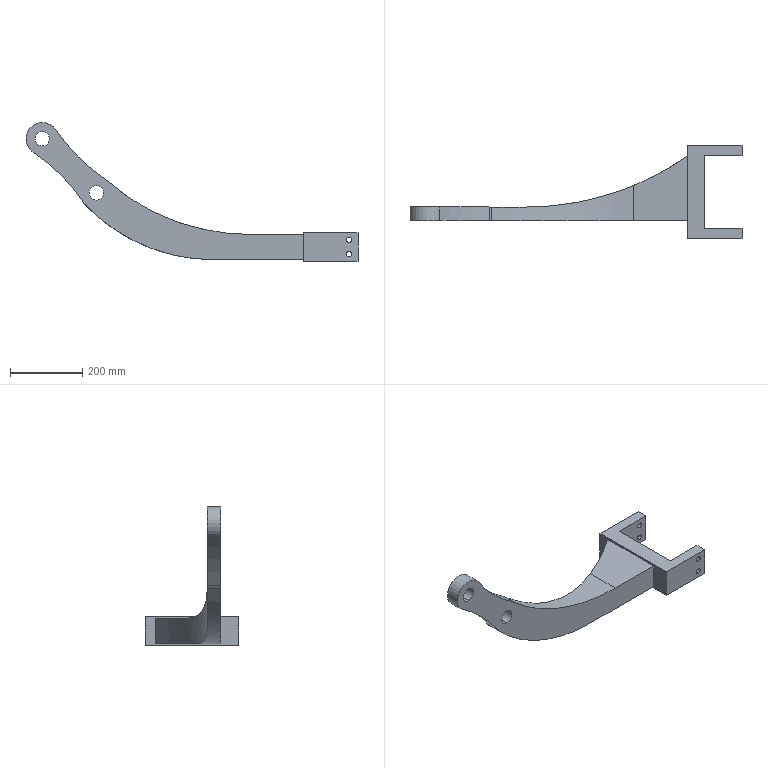Part | SolidWorks | features ICE 3, Cut 1, Extrusion 1, MirrorSolid 1 | 1 solid | 34 faces | box 920 x 260 x 385 mm | volume 5479591 mm3 | cylinder 20 | plane 14 | commonest cylinder face diameters 15 x8 40 x4 90 x3 1000 x2 984.464 x1 1199 x1
STEP:
#1=CARTESIAN_POINT('',(50.,-130.,12.5));
#2=VERTEX_POINT('',#1);
#3=CARTESIAN_POINT('',(50.,-130.,27.5));
#4=VERTEX_POINT('',#3);
#5=CARTESIAN_POINT('',(50.,-130.,20.));
#6=DIRECTION('',(0.,-1.,0.));
#7=DIRECTION('',(0.,0.,-1.));
#8=AXIS2_PLACEMENT_3D('',#5,#6,#7);
#9=CIRCLE('',#8,7.5);
#10=EDGE_CURVE('',#2,#4,#9,.T.);
#11=ORIENTED_EDGE('',*,*,#10,.T.);
#12=CARTESIAN_POINT('',(50.,-100.,27.5));
#13=VERTEX_POINT('',#12);
#14=CARTESIAN_POINT('',(50.,-130.,27.5));
#15=DIRECTION('',(0.,1.,0.));
#16=VECTOR('',#15,1000.);
#17=LINE('',#14,#16);
#18=EDGE_CURVE('',#4,#13,#17,.T.);
#19=ORIENTED_EDGE('',*,*,#18,.T.);
#20=CARTESIAN_POINT('',(50.,-100.,12.5));
#21=VERTEX_POINT('',#20);
#22=CARTESIAN_POINT('',(50.,-100.,20.));
#23=DIRECTION('',(0.,1.,0.));
#24=DIRECTION('',(0.,0.,1.));
#25=AXIS2_PLACEMENT_3D('',#22,#23,#24);
#26=CIRCLE('',#25,7.5);
#27=EDGE_CURVE('',#13,#21,#26,.T.);
#28=ORIENTED_EDGE('',*,*,#27,.T.);
#29=CARTESIAN_POINT('',(50.,-130.,12.5));
#30=DIRECTION('',(0.,1.,0.));
#31=VECTOR('',#30,1000.);
#32=LINE('',#29,#31);
#33=EDGE_CURVE('',#2,#21,#32,.T.);
#34=ORIENTED_EDGE('',*,*,#33,.F.);
#35=EDGE_LOOP('',(#11,#19,#28,#34));
#36=FACE_OUTER_BOUND('',#35,.T.);
#37=CARTESIAN_POINT('',(50.,-130.,20.));
#38=DIRECTION('',(0.,1.,0.));
#39=DIRECTION('',(0.,0.,-1.));
#40=AXIS2_PLACEMENT_3D('',#37,#38,#39);
#41=CYLINDRICAL_SURFACE('',#40,7.5);
#42=ADVANCED_FACE('',(#36),#41,.F.);
#43=CARTESIAN_POINT('',(50.,-130.,-27.5));
#44=VERTEX_POINT('',#43);
#45=CARTESIAN_POINT('',(50.,-130.,-12.5));
#46=VERTEX_POINT('',#45);
#47=CARTESIAN_POINT('',(50.,-130.,-20.));
#48=DIRECTION('',(0.,-1.,0.));
#49=DIRECTION('',(0.,0.,-1.));
#50=AXIS2_PLACEMENT_3D('',#47,#48,#49);
#51=CIRCLE('',#50,7.5);
#52=EDGE_CURVE('',#44,#46,#51,.T.);
#53=ORIENTED_EDGE('',*,*,#52,.T.);
#54=CARTESIAN_POINT('',(50.,-100.,-12.5));
#55=VERTEX_POINT('',#54);
#56=CARTESIAN_POINT('',(50.,-130.,-12.5));
#57=DIRECTION('',(0.,1.,0.));
#58=VECTOR('',#57,1000.);
#59=LINE('',#56,#58);
#60=EDGE_CURVE('',#46,#55,#59,.T.);
#61=ORIENTED_EDGE('',*,*,#60,.T.);
#62=CARTESIAN_POINT('',(50.,-100.,-27.5));
#63=VERTEX_POINT('',#62);
#64=CARTESIAN_POINT('',(50.,-100.,-20.));
#65=DIRECTION('',(0.,1.,0.));
#66=DIRECTION('',(0.,0.,1.));
#67=AXIS2_PLACEMENT_3D('',#64,#65,#66);
#68=CIRCLE('',#67,7.5);
#69=EDGE_CURVE('',#55,#63,#68,.T.);
#70=ORIENTED_EDGE('',*,*,#69,.T.);
#71=CARTESIAN_POINT('',(50.,-130.,-27.5));
#72=DIRECTION('',(0.,1.,0.));
#73=VECTOR('',#72,1000.);
#74=LINE('',#71,#73);
#75=EDGE_CURVE('',#44,#63,#74,.T.);
#76=ORIENTED_EDGE('',*,*,#75,.F.);
#77=EDGE_LOOP('',(#53,#61,#70,#76));
#78=FACE_OUTER_BOUND('',#77,.T.);
#79=CARTESIAN_POINT('',(50.,-130.,-20.));
#80=DIRECTION('',(0.,1.,0.));
#81=DIRECTION('',(0.,0.,-1.));
#82=AXIS2_PLACEMENT_3D('',#79,#80,#81);
#83=CYLINDRICAL_SURFACE('',#82,7.5);
#84=ADVANCED_FACE('',(#78),#83,.F.);
#85=CARTESIAN_POINT('',(50.,100.,12.5));
#86=VERTEX_POINT('',#85);
#87=CARTESIAN_POINT('',(50.,100.,27.5));
#88=VERTEX_POINT('',#87);
#89=CARTESIAN_POINT('',(50.,100.,20.));
#90=DIRECTION('',(0.,-1.,0.));
#91=DIRECTION('',(0.,0.,-1.));
#92=AXIS2_PLACEMENT_3D('',#89,#90,#91);
#93=CIRCLE('',#92,7.5);
#94=EDGE_CURVE('',#86,#88,#93,.T.);
#95=ORIENTED_EDGE('',*,*,#94,.T.);
#96=CARTESIAN_POINT('',(50.,130.,27.5));
#97=VERTEX_POINT('',#96);
#98=CARTESIAN_POINT('',(50.,-130.,27.5));
#99=DIRECTION('',(0.,1.,0.));
#100=VECTOR('',#99,1000.);
#101=LINE('',#98,#100);
#102=EDGE_CURVE('',#88,#97,#101,.T.);
#103=ORIENTED_EDGE('',*,*,#102,.T.);
#104=CARTESIAN_POINT('',(50.,130.,12.5));
#105=VERTEX_POINT('',#104);
#106=CARTESIAN_POINT('',(50.,130.,20.));
#107=DIRECTION('',(0.,-1.,0.));
#108=DIRECTION('',(0.,0.,-1.));
#109=AXIS2_PLACEMENT_3D('',#106,#107,#108);
#110=CIRCLE('',#109,7.5);
#111=EDGE_CURVE('',#105,#97,#110,.T.);
#112=ORIENTED_EDGE('',*,*,#111,.F.);
#113=CARTESIAN_POINT('',(50.,-130.,12.5));
#114=DIRECTION('',(0.,1.,0.));
#115=VECTOR('',#114,1000.);
#116=LINE('',#113,#115);
#117=EDGE_CURVE('',#86,#105,#116,.T.);
#118=ORIENTED_EDGE('',*,*,#117,.F.);
#119=EDGE_LOOP('',(#95,#103,#112,#118));
#120=FACE_OUTER_BOUND('',#119,.T.);
#121=CARTESIAN_POINT('',(50.,-130.,20.));
#122=DIRECTION('',(0.,1.,0.));
#123=DIRECTION('',(0.,0.,-1.));
#124=AXIS2_PLACEMENT_3D('',#121,#122,#123);
#125=CYLINDRICAL_SURFACE('',#124,7.5);
#126=ADVANCED_FACE('',(#120),#125,.F.);
#127=CARTESIAN_POINT('',(50.,100.,-27.5));
#128=VERTEX_POINT('',#127);
#129=CARTESIAN_POINT('',(50.,100.,-12.5));
#130=VERTEX_POINT('',#129);
#131=CARTESIAN_POINT('',(50.,100.,-20.));
#132=DIRECTION('',(0.,-1.,0.));
#133=DIRECTION('',(0.,0.,-1.));
#134=AXIS2_PLACEMENT_3D('',#131,#132,#133);
#135=CIRCLE('',#134,7.5);
#136=EDGE_CURVE('',#128,#130,#135,.T.);
#137=ORIENTED_EDGE('',*,*,#136,.T.);
#138=CARTESIAN_POINT('',(50.,130.,-12.5));
#139=VERTEX_POINT('',#138);
#140=CARTESIAN_POINT('',(50.,-130.,-12.5));
#141=DIRECTION('',(0.,1.,0.));
#142=VECTOR('',#141,1000.);
#143=LINE('',#140,#142);
#144=EDGE_CURVE('',#130,#139,#143,.T.);
#145=ORIENTED_EDGE('',*,*,#144,.T.);
#146=CARTESIAN_POINT('',(50.,130.,-27.5));
#147=VERTEX_POINT('',#146);
#148=CARTESIAN_POINT('',(50.,130.,-20.));
#149=DIRECTION('',(0.,-1.,0.));
#150=DIRECTION('',(0.,0.,-1.));
#151=AXIS2_PLACEMENT_3D('',#148,#149,#150);
#152=CIRCLE('',#151,7.5);
#153=EDGE_CURVE('',#147,#139,#152,.T.);
#154=ORIENTED_EDGE('',*,*,#153,.F.);
#155=CARTESIAN_POINT('',(50.,-130.,-27.5));
#156=DIRECTION('',(0.,1.,0.));
#157=VECTOR('',#156,1000.);
#158=LINE('',#155,#157);
#159=EDGE_CURVE('',#128,#147,#158,.T.);
#160=ORIENTED_EDGE('',*,*,#159,.F.);
#161=EDGE_LOOP('',(#137,#145,#154,#160));
#162=FACE_OUTER_BOUND('',#161,.T.);
#163=CARTESIAN_POINT('',(50.,-130.,-20.));
#164=DIRECTION('',(0.,1.,0.));
#165=DIRECTION('',(0.,0.,-1.));
#166=AXIS2_PLACEMENT_3D('',#163,#164,#165);
#167=CYLINDRICAL_SURFACE('',#166,7.5);
#168=ADVANCED_FACE('',(#162),#167,.F.);
#169=CARTESIAN_POINT('',(-650.,-80.,170.));
#170=VERTEX_POINT('',#169);
#171=CARTESIAN_POINT('',(-650.,-80.,130.));
#172=VERTEX_POINT('',#171);
#173=CARTESIAN_POINT('',(-650.,-80.,150.));
#174=DIRECTION('',(0.,1.,0.));
#175=DIRECTION('',(-1.,0.,0.));
#176=AXIS2_PLACEMENT_3D('',#173,#174,#175);
#177=CIRCLE('',#176,20.);
#178=EDGE_CURVE('',#170,#172,#177,.T.);
#179=ORIENTED_EDGE('',*,*,#178,.F.);
#180=CARTESIAN_POINT('',(-650.,-41.894,170.));
#181=VERTEX_POINT('',#180);
#182=CARTESIAN_POINT('',(-650.,-100.,170.));
#183=DIRECTION('',(0.,1.,0.));
#184=VECTOR('',#183,1000.);
#185=LINE('',#182,#184);
#186=EDGE_CURVE('',#170,#181,#185,.T.);
#187=ORIENTED_EDGE('',*,*,#186,.T.);
#188=CARTESIAN_POINT('',(-650.,-41.894,130.));
#189=VERTEX_POINT('',#188);
#190=CARTESIAN_POINT('',(-650.,-41.894,150.));
#191=DIRECTION('',(0.,-1.,0.));
#192=DIRECTION('',(0.,0.,1.));
#193=AXIS2_PLACEMENT_3D('',#190,#191,#192);
#194=CIRCLE('',#193,20.);
#195=EDGE_CURVE('',#189,#181,#194,.T.);
#196=ORIENTED_EDGE('',*,*,#195,.F.);
#197=CARTESIAN_POINT('',(-650.,-100.,130.));
#198=DIRECTION('',(0.,1.,0.));
#199=VECTOR('',#198,1000.);
#200=LINE('',#197,#199);
#201=EDGE_CURVE('',#172,#189,#200,.T.);
#202=ORIENTED_EDGE('',*,*,#201,.F.);
#203=EDGE_LOOP('',(#179,#187,#196,#202));
#204=FACE_OUTER_BOUND('',#203,.T.);
#205=CARTESIAN_POINT('',(-650.,-100.,150.));
#206=DIRECTION('',(0.,1.,0.));
#207=DIRECTION('',(0.,0.,-1.));
#208=AXIS2_PLACEMENT_3D('',#205,#206,#207);
#209=CYLINDRICAL_SURFACE('',#208,20.);
#210=ADVANCED_FACE('',(#204),#209,.F.);
#211=CARTESIAN_POINT('',(-800.,-80.,320.));
#212=VERTEX_POINT('',#211);
#213=CARTESIAN_POINT('',(-800.,-80.,280.));
#214=VERTEX_POINT('',#213);
#215=CARTESIAN_POINT('',(-800.,-80.,300.));
#216=DIRECTION('',(0.,1.,0.));
#217=DIRECTION('',(-1.,0.,0.));
#218=AXIS2_PLACEMENT_3D('',#215,#216,#217);
#219=CIRCLE('',#218,20.);
#220=EDGE_CURVE('',#212,#214,#219,.T.);
#221=ORIENTED_EDGE('',*,*,#220,.F.);
#222=CARTESIAN_POINT('',(-800.,-41.894,320.));
#223=VERTEX_POINT('',#222);
#224=CARTESIAN_POINT('',(-800.,-100.,320.));
#225=DIRECTION('',(0.,1.,0.));
#226=VECTOR('',#225,1000.);
#227=LINE('',#224,#226);
#228=EDGE_CURVE('',#212,#223,#227,.T.);
#229=ORIENTED_EDGE('',*,*,#228,.T.);
#230=CARTESIAN_POINT('',(-800.,-41.894,280.));
#231=VERTEX_POINT('',#230);
#232=CARTESIAN_POINT('',(-800.,-41.894,300.));
#233=DIRECTION('',(0.,-1.,0.));
#234=DIRECTION('',(0.,0.,1.));
#235=AXIS2_PLACEMENT_3D('',#232,#233,#234);
#236=CIRCLE('',#235,20.);
#237=EDGE_CURVE('',#231,#223,#236,.T.);
#238=ORIENTED_EDGE('',*,*,#237,.F.);
#239=CARTESIAN_POINT('',(-800.,-100.,280.));
#240=DIRECTION('',(0.,1.,0.));
#241=VECTOR('',#240,1000.);
#242=LINE('',#239,#241);
#243=EDGE_CURVE('',#214,#231,#242,.T.);
#244=ORIENTED_EDGE('',*,*,#243,.F.);
#245=EDGE_LOOP('',(#221,#229,#238,#244));
#246=FACE_OUTER_BOUND('',#245,.T.);
#247=CARTESIAN_POINT('',(-800.,-100.,300.));
#248=DIRECTION('',(0.,1.,0.));
#249=DIRECTION('',(0.,0.,-1.));
#250=AXIS2_PLACEMENT_3D('',#247,#248,#249);
#251=CYLINDRICAL_SURFACE('',#250,20.);
#252=ADVANCED_FACE('',(#246),#251,.F.);
#253=CARTESIAN_POINT('',(-75.,100.,-35.));
#254=VERTEX_POINT('',#253);
#255=CARTESIAN_POINT('',(-75.,100.,35.));
#256=VERTEX_POINT('',#255);
#257=CARTESIAN_POINT('',(-75.,100.,35.));
#258=DIRECTION('',(0.,0.,1.));
#259=VECTOR('',#258,1000.);
#260=LINE('',#257,#259);
#261=EDGE_CURVE('',#254,#256,#260,.T.);
#262=ORIENTED_EDGE('',*,*,#261,.T.);
#263=CARTESIAN_POINT('',(-75.,-80.,35.));
#264=VERTEX_POINT('',#263);
#265=CARTESIAN_POINT('',(-75.,-100.,35.));
#266=DIRECTION('',(0.,1.,0.));
#267=VECTOR('',#266,1000.);
#268=LINE('',#265,#267);
#269=EDGE_CURVE('',#264,#256,#268,.T.);
#270=ORIENTED_EDGE('',*,*,#269,.F.);
#271=CARTESIAN_POINT('',(-75.,-80.,-35.));
#272=VERTEX_POINT('',#271);
#273=CARTESIAN_POINT('',(-75.,-80.,345.));
#274=DIRECTION('',(0.,0.,-1.));
#275=VECTOR('',#274,1000.);
#276=LINE('',#273,#275);
#277=EDGE_CURVE('',#264,#272,#276,.T.);
#278=ORIENTED_EDGE('',*,*,#277,.T.);
#279=CARTESIAN_POINT('',(-75.,-100.,-35.));
#280=DIRECTION('',(0.,1.,0.));
#281=VECTOR('',#280,1000.);
#282=LINE('',#279,#281);
#283=EDGE_CURVE('',#272,#254,#282,.T.);
#284=ORIENTED_EDGE('',*,*,#283,.T.);
#285=EDGE_LOOP('',(#262,#270,#278,#284));
#286=FACE_BOUND('',#285,.T.);
#287=CARTESIAN_POINT('',(-75.,130.,40.));
#288=VERTEX_POINT('',#287);
#289=CARTESIAN_POINT('',(-75.,-130.,40.));
#290=VERTEX_POINT('',#289);
#291=CARTESIAN_POINT('',(-75.,130.,40.));
#292=DIRECTION('',(0.,-1.,0.));
#293=VECTOR('',#292,1000.);
#294=LINE('',#291,#293);
#295=EDGE_CURVE('',#288,#290,#294,.T.);
#296=ORIENTED_EDGE('',*,*,#295,.F.);
#297=CARTESIAN_POINT('',(-75.,130.,-40.));
#298=VERTEX_POINT('',#297);
#299=CARTESIAN_POINT('',(-75.,130.,-40.));
#300=DIRECTION('',(0.,0.,1.));
#301=VECTOR('',#300,1000.);
#302=LINE('',#299,#301);
#303=EDGE_CURVE('',#298,#288,#302,.T.);
#304=ORIENTED_EDGE('',*,*,#303,.F.);
#305=CARTESIAN_POINT('',(-75.,-130.,-40.));
#306=VERTEX_POINT('',#305);
#307=CARTESIAN_POINT('',(-75.,130.,-40.));
#308=DIRECTION('',(0.,-1.,0.));
#309=VECTOR('',#308,1000.);
#310=LINE('',#307,#309);
#311=EDGE_CURVE('',#298,#306,#310,.T.);
#312=ORIENTED_EDGE('',*,*,#311,.T.);
#313=CARTESIAN_POINT('',(-75.,-130.,-40.));
#314=DIRECTION('',(0.,0.,1.));
#315=VECTOR('',#314,1000.);
#316=LINE('',#313,#315);
#317=EDGE_CURVE('',#306,#290,#316,.T.);
#318=ORIENTED_EDGE('',*,*,#317,.T.);
#319=EDGE_LOOP('',(#296,#304,#312,#318));
#320=FACE_OUTER_BOUND('',#319,.T.);
#321=CARTESIAN_POINT('',(-75.,130.,-40.));
#322=DIRECTION('',(1.,0.,0.));
#323=DIRECTION('',(0.,1.,0.));
#324=AXIS2_PLACEMENT_3D('',#321,#322,#323);
#325=PLANE('',#324);
#326=ADVANCED_FACE('',(#286,#320),#325,.F.);
#327=CARTESIAN_POINT('',(75.,-130.,40.));
#328=VERTEX_POINT('',#327);
#329=CARTESIAN_POINT('',(75.,-100.,40.));
#330=VERTEX_POINT('',#329);
#331=CARTESIAN_POINT('',(75.,130.,40.));
#332=DIRECTION('',(0.,1.,0.));
#333=VECTOR('',#332,1000.);
#334=LINE('',#331,#333);
#335=EDGE_CURVE('',#328,#330,#334,.T.);
#336=ORIENTED_EDGE('',*,*,#335,.F.);
#337=CARTESIAN_POINT('',(75.,-130.,-40.));
#338=VERTEX_POINT('',#337);
#339=CARTESIAN_POINT('',(75.,-130.,-40.));
#340=DIRECTION('',(0.,0.,1.));
#341=VECTOR('',#340,1000.);
#342=LINE('',#339,#341);
#343=EDGE_CURVE('',#338,#328,#342,.T.);
#344=ORIENTED_EDGE('',*,*,#343,.F.);
#345=CARTESIAN_POINT('',(75.,-100.,-40.));
#346=VERTEX_POINT('',#345);
#347=CARTESIAN_POINT('',(75.,130.,-40.));
#348=DIRECTION('',(0.,1.,0.));
#349=VECTOR('',#348,1000.);
#350=LINE('',#347,#349);
#351=EDGE_CURVE('',#338,#346,#350,.T.);
#352=ORIENTED_EDGE('',*,*,#351,.T.);
#353=CARTESIAN_POINT('',(75.,-100.,-40.));
#354=DIRECTION('',(0.,0.,-1.));
#355=VECTOR('',#354,1000.);
#356=LINE('',#353,#355);
#357=EDGE_CURVE('',#330,#346,#356,.T.);
#358=ORIENTED_EDGE('',*,*,#357,.F.);
#359=EDGE_LOOP('',(#336,#344,#352,#358));
#360=FACE_OUTER_BOUND('',#359,.T.);
#361=CARTESIAN_POINT('',(75.,130.,-40.));
#362=DIRECTION('',(-1.,0.,0.));
#363=DIRECTION('',(0.,-1.,0.));
#364=AXIS2_PLACEMENT_3D('',#361,#362,#363);
#365=PLANE('',#364);
#366=ADVANCED_FACE('',(#360),#365,.F.);
#367=CARTESIAN_POINT('',(75.,100.,-40.));
#368=VERTEX_POINT('',#367);
#369=CARTESIAN_POINT('',(75.,130.,-40.));
#370=VERTEX_POINT('',#369);
#371=CARTESIAN_POINT('',(75.,130.,-40.));
#372=DIRECTION('',(0.,1.,0.));
#373=VECTOR('',#372,1000.);
#374=LINE('',#371,#373);
#375=EDGE_CURVE('',#368,#370,#374,.T.);
#376=ORIENTED_EDGE('',*,*,#375,.T.);
#377=CARTESIAN_POINT('',(75.,130.,40.));
#378=VERTEX_POINT('',#377);
#379=CARTESIAN_POINT('',(75.,130.,-40.));
#380=DIRECTION('',(0.,0.,1.));
#381=VECTOR('',#380,1000.);
#382=LINE('',#379,#381);
#383=EDGE_CURVE('',#370,#378,#382,.T.);
#384=ORIENTED_EDGE('',*,*,#383,.T.);
#385=CARTESIAN_POINT('',(75.,100.,40.));
#386=VERTEX_POINT('',#385);
#387=CARTESIAN_POINT('',(75.,130.,40.));
#388=DIRECTION('',(0.,1.,0.));
#389=VECTOR('',#388,1000.);
#390=LINE('',#387,#389);
#391=EDGE_CURVE('',#386,#378,#390,.T.);
#392=ORIENTED_EDGE('',*,*,#391,.F.);
#393=CARTESIAN_POINT('',(75.,100.,-40.));
#394=DIRECTION('',(0.,0.,1.));
#395=VECTOR('',#394,1000.);
#396=LINE('',#393,#395);
#397=EDGE_CURVE('',#368,#386,#396,.T.);
#398=ORIENTED_EDGE('',*,*,#397,.F.);
#399=EDGE_LOOP('',(#376,#384,#392,#398));
#400=FACE_OUTER_BOUND('',#399,.T.);
#401=CARTESIAN_POINT('',(75.,130.,-40.));
#402=DIRECTION('',(-1.,0.,0.));
#403=DIRECTION('',(0.,-1.,0.));
#404=AXIS2_PLACEMENT_3D('',#401,#402,#403);
#405=PLANE('',#404);
#406=ADVANCED_FACE('',(#400),#405,.F.);
#407=ORIENTED_EDGE('',*,*,#111,.T.);
#408=CARTESIAN_POINT('',(50.,130.,20.));
#409=DIRECTION('',(0.,-1.,0.));
#410=DIRECTION('',(0.,0.,-1.));
#411=AXIS2_PLACEMENT_3D('',#408,#409,#410);
#412=CIRCLE('',#411,7.5);
#413=EDGE_CURVE('',#97,#105,#412,.T.);
#414=ORIENTED_EDGE('',*,*,#413,.T.);
#415=EDGE_LOOP('',(#407,#414));
#416=FACE_BOUND('',#415,.T.);
#417=ORIENTED_EDGE('',*,*,#153,.T.);
#418=CARTESIAN_POINT('',(50.,130.,-20.));
#419=DIRECTION('',(0.,-1.,0.));
#420=DIRECTION('',(0.,0.,-1.));
#421=AXIS2_PLACEMENT_3D('',#418,#419,#420);
#422=CIRCLE('',#421,7.5);
#423=EDGE_CURVE('',#139,#147,#422,.T.);
#424=ORIENTED_EDGE('',*,*,#423,.T.);
#425=EDGE_LOOP('',(#417,#424));
#426=FACE_BOUND('',#425,.T.);
#427=CARTESIAN_POINT('',(-75.,130.,40.));
#428=DIRECTION('',(-1.,0.,0.));
#429=VECTOR('',#428,1000.);
#430=LINE('',#427,#429);
#431=EDGE_CURVE('',#378,#288,#430,.T.);
#432=ORIENTED_EDGE('',*,*,#431,.F.);
#433=ORIENTED_EDGE('',*,*,#383,.F.);
#434=CARTESIAN_POINT('',(-75.,130.,-40.));
#435=DIRECTION('',(-1.,0.,0.));
#436=VECTOR('',#435,1000.);
#437=LINE('',#434,#436);
#438=EDGE_CURVE('',#370,#298,#437,.T.);
#439=ORIENTED_EDGE('',*,*,#438,.T.);
#440=ORIENTED_EDGE('',*,*,#303,.T.);
#441=EDGE_LOOP('',(#432,#433,#439,#440));
#442=FACE_OUTER_BOUND('',#441,.T.);
#443=CARTESIAN_POINT('',(-75.,130.,-40.));
#444=DIRECTION('',(0.,-1.,0.));
#445=DIRECTION('',(0.,0.,1.));
#446=AXIS2_PLACEMENT_3D('',#443,#444,#445);
#447=PLANE('',#446);
#448=ADVANCED_FACE('',(#416,#426,#442),#447,.F.);
#449=ORIENTED_EDGE('',*,*,#10,.F.);
#450=CARTESIAN_POINT('',(50.,-130.,20.));
#451=DIRECTION('',(0.,-1.,0.));
#452=DIRECTION('',(0.,0.,-1.));
#453=AXIS2_PLACEMENT_3D('',#450,#451,#452);
#454=CIRCLE('',#453,7.5);
#455=EDGE_CURVE('',#4,#2,#454,.T.);
#456=ORIENTED_EDGE('',*,*,#455,.F.);
#457=EDGE_LOOP('',(#449,#456));
#458=FACE_BOUND('',#457,.T.);
#459=ORIENTED_EDGE('',*,*,#52,.F.);
#460=CARTESIAN_POINT('',(50.,-130.,-20.));
#461=DIRECTION('',(0.,-1.,0.));
#462=DIRECTION('',(0.,0.,-1.));
#463=AXIS2_PLACEMENT_3D('',#460,#461,#462);
#464=CIRCLE('',#463,7.5);
#465=EDGE_CURVE('',#46,#44,#464,.T.);
#466=ORIENTED_EDGE('',*,*,#465,.F.);
#467=EDGE_LOOP('',(#459,#466));
#468=FACE_BOUND('',#467,.T.);
#469=CARTESIAN_POINT('',(-75.,-130.,40.));
#470=DIRECTION('',(1.,0.,0.));
#471=VECTOR('',#470,1000.);
#472=LINE('',#469,#471);
#473=EDGE_CURVE('',#290,#328,#472,.T.);
#474=ORIENTED_EDGE('',*,*,#473,.F.);
#475=ORIENTED_EDGE('',*,*,#317,.F.);
#476=CARTESIAN_POINT('',(-75.,-130.,-40.));
#477=DIRECTION('',(1.,0.,0.));
#478=VECTOR('',#477,1000.);
#479=LINE('',#476,#478);
#480=EDGE_CURVE('',#306,#338,#479,.T.);
#481=ORIENTED_EDGE('',*,*,#480,.T.);
#482=ORIENTED_EDGE('',*,*,#343,.T.);
#483=EDGE_LOOP('',(#474,#475,#481,#482));
#484=FACE_OUTER_BOUND('',#483,.T.);
#485=CARTESIAN_POINT('',(-75.,-130.,-40.));
#486=DIRECTION('',(0.,1.,0.));
#487=DIRECTION('',(0.,0.,-1.));
#488=AXIS2_PLACEMENT_3D('',#485,#486,#487);
#489=PLANE('',#488);
#490=ADVANCED_FACE('',(#458,#468,#484),#489,.F.);
#491=CARTESIAN_POINT('',(-30.,-100.,-40.));
#492=VERTEX_POINT('',#491);
#493=CARTESIAN_POINT('',(-30.,-100.,-40.));
#494=DIRECTION('',(1.,0.,0.));
#495=VECTOR('',#494,1000.);
#496=LINE('',#493,#495);
#497=EDGE_CURVE('',#492,#346,#496,.T.);
#498=ORIENTED_EDGE('',*,*,#497,.T.);
#499=ORIENTED_EDGE('',*,*,#351,.F.);
#500=ORIENTED_EDGE('',*,*,#480,.F.);
#501=ORIENTED_EDGE('',*,*,#311,.F.);
#502=ORIENTED_EDGE('',*,*,#438,.F.);
#503=ORIENTED_EDGE('',*,*,#375,.F.);
#504=CARTESIAN_POINT('',(-30.,100.,-40.));
#505=VERTEX_POINT('',#504);
#506=CARTESIAN_POINT('',(-30.,100.,-40.));
#507=DIRECTION('',(-1.,0.,0.));
#508=VECTOR('',#507,1000.);
#509=LINE('',#506,#508);
#510=EDGE_CURVE('',#368,#505,#509,.T.);
#511=ORIENTED_EDGE('',*,*,#510,.T.);
#512=CARTESIAN_POINT('',(-30.,100.,-40.));
#513=DIRECTION('',(0.,-1.,0.));
#514=VECTOR('',#513,1000.);
#515=LINE('',#512,#514);
#516=EDGE_CURVE('',#505,#492,#515,.T.);
#517=ORIENTED_EDGE('',*,*,#516,.T.);
#518=EDGE_LOOP('',(#498,#499,#500,#501,#502,#503,#511,#517));
#519=FACE_OUTER_BOUND('',#518,.T.);
#520=CARTESIAN_POINT('',(0.,0.,-40.));
#521=DIRECTION('',(0.,0.,-1.));
#522=DIRECTION('',(1.,0.,0.));
#523=AXIS2_PLACEMENT_3D('',#520,#521,#522);
#524=PLANE('',#523);
#525=ADVANCED_FACE('',(#519),#524,.T.);
#526=CARTESIAN_POINT('',(-30.,100.,40.));
#527=VERTEX_POINT('',#526);
#528=CARTESIAN_POINT('',(-30.,-100.,40.));
#529=VERTEX_POINT('',#528);
#530=CARTESIAN_POINT('',(-30.,100.,40.));
#531=DIRECTION('',(0.,-1.,0.));
#532=VECTOR('',#531,1000.);
#533=LINE('',#530,#532);
#534=EDGE_CURVE('',#527,#529,#533,.T.);
#535=ORIENTED_EDGE('',*,*,#534,.F.);
#536=CARTESIAN_POINT('',(0.,100.,40.));
#537=DIRECTION('',(-1.,0.,0.));
#538=VECTOR('',#537,1000.);
#539=LINE('',#536,#538);
#540=EDGE_CURVE('',#386,#527,#539,.T.);
#541=ORIENTED_EDGE('',*,*,#540,.F.);
#542=ORIENTED_EDGE('',*,*,#391,.T.);
#543=ORIENTED_EDGE('',*,*,#431,.T.);
#544=ORIENTED_EDGE('',*,*,#295,.T.);
#545=ORIENTED_EDGE('',*,*,#473,.T.);
#546=ORIENTED_EDGE('',*,*,#335,.T.);
#547=CARTESIAN_POINT('',(-30.,-100.,40.));
#548=DIRECTION('',(1.,0.,0.));
#549=VECTOR('',#548,1000.);
#550=LINE('',#547,#549);
#551=EDGE_CURVE('',#529,#330,#550,.T.);
#552=ORIENTED_EDGE('',*,*,#551,.F.);
#553=EDGE_LOOP('',(#535,#541,#542,#543,#544,#545,#546,#552));
#554=FACE_OUTER_BOUND('',#553,.T.);
#555=CARTESIAN_POINT('',(0.,0.,40.));
#556=DIRECTION('',(0.,0.,-1.));
#557=DIRECTION('',(1.,0.,0.));
#558=AXIS2_PLACEMENT_3D('',#555,#556,#557);
#559=PLANE('',#558);
#560=ADVANCED_FACE('',(#554),#559,.F.);
#561=CARTESIAN_POINT('',(50.,-100.,20.));
#562=DIRECTION('',(0.,1.,0.));
#563=DIRECTION('',(0.,0.,1.));
#564=AXIS2_PLACEMENT_3D('',#561,#562,#563);
#565=CIRCLE('',#564,7.5);
#566=EDGE_CURVE('',#21,#13,#565,.T.);
#567=ORIENTED_EDGE('',*,*,#566,.F.);
#568=ORIENTED_EDGE('',*,*,#27,.F.);
#569=EDGE_LOOP('',(#567,#568));
#570=FACE_BOUND('',#569,.T.);
#571=CARTESIAN_POINT('',(50.,-100.,-20.));
#572=DIRECTION('',(0.,1.,0.));
#573=DIRECTION('',(0.,0.,1.));
#574=AXIS2_PLACEMENT_3D('',#571,#572,#573);
#575=CIRCLE('',#574,7.5);
#576=EDGE_CURVE('',#63,#55,#575,.T.);
#577=ORIENTED_EDGE('',*,*,#576,.F.);
#578=ORIENTED_EDGE('',*,*,#69,.F.);
#579=EDGE_LOOP('',(#577,#578));
#580=FACE_BOUND('',#579,.T.);
#581=ORIENTED_EDGE('',*,*,#551,.T.);
#582=ORIENTED_EDGE('',*,*,#357,.T.);
#583=ORIENTED_EDGE('',*,*,#497,.F.);
#584=CARTESIAN_POINT('',(-30.,-100.,40.));
#585=DIRECTION('',(0.,0.,-1.));
#586=VECTOR('',#585,1000.);
#587=LINE('',#584,#586);
#588=EDGE_CURVE('',#529,#492,#587,.T.);
#589=ORIENTED_EDGE('',*,*,#588,.F.);
#590=EDGE_LOOP('',(#581,#582,#583,#589));
#591=FACE_OUTER_BOUND('',#590,.T.);
#592=CARTESIAN_POINT('',(-30.,-100.,40.));
#593=DIRECTION('',(0.,-1.,0.));
#594=DIRECTION('',(0.,0.,1.));
#595=AXIS2_PLACEMENT_3D('',#592,#593,#594);
#596=PLANE('',#595);
#597=ADVANCED_FACE('',(#570,#580,#591),#596,.F.);
#598=ORIENTED_EDGE('',*,*,#94,.F.);
#599=CARTESIAN_POINT('',(50.,100.,20.));
#600=DIRECTION('',(0.,-1.,0.));
#601=DIRECTION('',(0.,0.,-1.));
#602=AXIS2_PLACEMENT_3D('',#599,#600,#601);
#603=CIRCLE('',#602,7.5);
#604=EDGE_CURVE('',#88,#86,#603,.T.);
#605=ORIENTED_EDGE('',*,*,#604,.F.);
#606=EDGE_LOOP('',(#598,#605));
#607=FACE_BOUND('',#606,.T.);
#608=ORIENTED_EDGE('',*,*,#136,.F.);
#609=CARTESIAN_POINT('',(50.,100.,-20.));
#610=DIRECTION('',(0.,-1.,0.));
#611=DIRECTION('',(0.,0.,-1.));
#612=AXIS2_PLACEMENT_3D('',#609,#610,#611);
#613=CIRCLE('',#612,7.5);
#614=EDGE_CURVE('',#130,#128,#613,.T.);
#615=ORIENTED_EDGE('',*,*,#614,.F.);
#616=EDGE_LOOP('',(#608,#615));
#617=FACE_BOUND('',#616,.T.);
#618=ORIENTED_EDGE('',*,*,#510,.F.);
#619=ORIENTED_EDGE('',*,*,#397,.T.);
#620=ORIENTED_EDGE('',*,*,#540,.T.);
#621=CARTESIAN_POINT('',(-30.,100.,40.));
#622=DIRECTION('',(0.,0.,-1.));
#623=VECTOR('',#622,1000.);
#624=LINE('',#621,#623);
#625=EDGE_CURVE('',#527,#505,#624,.T.);
#626=ORIENTED_EDGE('',*,*,#625,.T.);
#627=EDGE_LOOP('',(#618,#619,#620,#626));
#628=FACE_OUTER_BOUND('',#627,.T.);
#629=CARTESIAN_POINT('',(-30.,100.,40.));
#630=DIRECTION('',(0.,1.,0.));
#631=DIRECTION('',(0.,0.,-1.));
#632=AXIS2_PLACEMENT_3D('',#629,#630,#631);
#633=PLANE('',#632);
#634=ADVANCED_FACE('',(#607,#617,#628),#633,.F.);
#635=ORIENTED_EDGE('',*,*,#516,.F.);
#636=ORIENTED_EDGE('',*,*,#625,.F.);
#637=ORIENTED_EDGE('',*,*,#534,.T.);
#638=ORIENTED_EDGE('',*,*,#588,.T.);
#639=EDGE_LOOP('',(#635,#636,#637,#638));
#640=FACE_OUTER_BOUND('',#639,.T.);
#641=CARTESIAN_POINT('',(-30.,100.,40.));
#642=DIRECTION('',(-1.,0.,0.));
#643=DIRECTION('',(0.,-1.,0.));
#644=AXIS2_PLACEMENT_3D('',#641,#642,#643);
#645=PLANE('',#644);
#646=ADVANCED_FACE('',(#640),#645,.F.);
#647=CARTESIAN_POINT('',(-225.,17.733,35.));
#648=VERTEX_POINT('',#647);
#649=CARTESIAN_POINT('',(-525.,742.612,35.));
#650=DIRECTION('',(0.,0.,-1.));
#651=DIRECTION('',(-1.,0.,0.));
#652=AXIS2_PLACEMENT_3D('',#649,#650,#651);
#653=CIRCLE('',#652,784.506);
#654=EDGE_CURVE('',#256,#648,#653,.T.);
#655=ORIENTED_EDGE('',*,*,#654,.T.);
#656=CARTESIAN_POINT('',(-225.,-80.,35.));
#657=VERTEX_POINT('',#656);
#658=CARTESIAN_POINT('',(-225.,-100.,35.));
#659=DIRECTION('',(0.,1.,0.));
#660=VECTOR('',#659,1000.);
#661=LINE('',#658,#660);
#662=EDGE_CURVE('',#657,#648,#661,.T.);
#663=ORIENTED_EDGE('',*,*,#662,.F.);
#664=CARTESIAN_POINT('',(-75.,-80.,35.));
#665=DIRECTION('',(1.,0.,0.));
#666=VECTOR('',#665,1000.);
#667=LINE('',#664,#666);
#668=EDGE_CURVE('',#657,#264,#667,.T.);
#669=ORIENTED_EDGE('',*,*,#668,.T.);
#670=ORIENTED_EDGE('',*,*,#269,.T.);
#671=EDGE_LOOP('',(#655,#663,#669,#670));
#672=FACE_OUTER_BOUND('',#671,.T.);
#673=CARTESIAN_POINT('',(-75.,-100.,35.));
#674=DIRECTION('',(0.,0.,1.));
#675=DIRECTION('',(-1.,0.,0.));
#676=AXIS2_PLACEMENT_3D('',#673,#674,#675);
#677=PLANE('',#676);
#678=ADVANCED_FACE('',(#672),#677,.T.);
#679=CARTESIAN_POINT('',(-325.,-15.972,-35.));
#680=VERTEX_POINT('',#679);
#681=CARTESIAN_POINT('',(-525.,742.612,-35.));
#682=DIRECTION('',(0.,0.,1.));
#683=DIRECTION('',(1.,0.,0.));
#684=AXIS2_PLACEMENT_3D('',#681,#682,#683);
#685=CIRCLE('',#684,784.506);
#686=EDGE_CURVE('',#680,#254,#685,.T.);
#687=ORIENTED_EDGE('',*,*,#686,.T.);
#688=ORIENTED_EDGE('',*,*,#283,.F.);
#689=CARTESIAN_POINT('',(-325.,-80.,-35.));
#690=VERTEX_POINT('',#689);
#691=CARTESIAN_POINT('',(-75.,-80.,-35.));
#692=DIRECTION('',(-1.,0.,0.));
#693=VECTOR('',#692,1000.);
#694=LINE('',#691,#693);
#695=EDGE_CURVE('',#272,#690,#694,.T.);
#696=ORIENTED_EDGE('',*,*,#695,.T.);
#697=CARTESIAN_POINT('',(-325.,-100.,-35.));
#698=DIRECTION('',(0.,1.,0.));
#699=VECTOR('',#698,1000.);
#700=LINE('',#697,#699);
#701=EDGE_CURVE('',#690,#680,#700,.T.);
#702=ORIENTED_EDGE('',*,*,#701,.T.);
#703=EDGE_LOOP('',(#687,#688,#696,#702));
#704=FACE_OUTER_BOUND('',#703,.T.);
#705=CARTESIAN_POINT('',(-75.,-100.,-35.));
#706=DIRECTION('',(0.,0.,-1.));
#707=DIRECTION('',(1.,0.,0.));
#708=AXIS2_PLACEMENT_3D('',#705,#706,#707);
#709=PLANE('',#708);
#710=ADVANCED_FACE('',(#704),#709,.T.);
#711=CARTESIAN_POINT('',(-525.,-41.894,7.463));
#712=VERTEX_POINT('',#711);
#713=CARTESIAN_POINT('',(-525.,-41.894,7.463));
#714=CARTESIAN_POINT('',(-517.108,-41.894,3.953));
#715=CARTESIAN_POINT('',(-509.105,-41.775,0.6434));
#716=CARTESIAN_POINT('',(-496.932,-41.403,-4.017));
#717=CARTESIAN_POINT('',(-492.846,-41.246,-5.52));
#718=CARTESIAN_POINT('',(-486.675,-40.96,-7.696));
#719=CARTESIAN_POINT('',(-484.61,-40.857,-8.409));
#720=CARTESIAN_POINT('',(-480.467,-40.632,-9.809));
#721=CARTESIAN_POINT('',(-478.387,-40.511,-10.496));
#722=CARTESIAN_POINT('',(-459.666,-39.347,-16.543));
#723=CARTESIAN_POINT('',(-442.957,-37.776,-20.964));
#724=CARTESIAN_POINT('',(-409.429,-33.519,-28.008));
#725=CARTESIAN_POINT('',(-392.608,-30.833,-30.63));
#726=CARTESIAN_POINT('',(-367.307,-25.93,-33.252));
#727=CARTESIAN_POINT('',(-358.861,-24.15,-33.907));
#728=CARTESIAN_POINT('',(-346.175,-21.254,-34.563));
#729=CARTESIAN_POINT('',(-341.944,-20.251,-34.727));
#730=CARTESIAN_POINT('',(-335.593,-18.689,-34.891));
#731=CARTESIAN_POINT('',(-333.475,-18.16,-34.932));
#732=CARTESIAN_POINT('',(-329.239,-17.08,-34.986));
#733=CARTESIAN_POINT('',(-327.118,-16.531,-35.));
#734=CARTESIAN_POINT('',(-325.,-15.972,-35.));
#735=B_SPLINE_CURVE_WITH_KNOTS('',3,(#713,#714,#715,#716,#717,#718,#719,#720,#721,#722,#723,#724,#725,#726,#727,#728,#729,#730,#731,#732,#733,#734),.UNSPECIFIED.,.F.,.F.,(4,2,2,2,2,2,2,2,2,2,4),(3.078,3.104,3.117,3.123,3.13,3.182,3.233,3.259,3.272,3.278,3.285),.UNSPECIFIED.);
#736=EDGE_CURVE('',#712,#680,#735,.T.);
#737=ORIENTED_EDGE('',*,*,#736,.T.);
#738=ORIENTED_EDGE('',*,*,#701,.F.);
#739=CARTESIAN_POINT('',(-682.701,-80.,119.087));
#740=VERTEX_POINT('',#739);
#741=CARTESIAN_POINT('',(-325.,-80.,457.232));
#742=DIRECTION('',(0.,1.,0.));
#743=DIRECTION('',(-1.,0.,0.));
#744=AXIS2_PLACEMENT_3D('',#741,#742,#743);
#745=CIRCLE('',#744,492.232);
#746=EDGE_CURVE('',#690,#740,#745,.T.);
#747=ORIENTED_EDGE('',*,*,#746,.T.);
#748=CARTESIAN_POINT('',(-682.701,-41.894,119.087));
#749=VERTEX_POINT('',#748);
#750=CARTESIAN_POINT('',(-682.701,-100.,119.087));
#751=DIRECTION('',(0.,1.,0.));
#752=VECTOR('',#751,1000.);
#753=LINE('',#750,#752);
#754=EDGE_CURVE('',#740,#749,#753,.T.);
#755=ORIENTED_EDGE('',*,*,#754,.T.);
#756=CARTESIAN_POINT('',(-325.,-41.894,457.232));
#757=DIRECTION('',(0.,-1.,0.));
#758=DIRECTION('',(0.,0.,1.));
#759=AXIS2_PLACEMENT_3D('',#756,#757,#758);
#760=CIRCLE('',#759,492.232);
#761=EDGE_CURVE('',#749,#712,#760,.T.);
#762=ORIENTED_EDGE('',*,*,#761,.T.);
#763=EDGE_LOOP('',(#737,#738,#747,#755,#762));
#764=FACE_OUTER_BOUND('',#763,.T.);
#765=CARTESIAN_POINT('',(-325.,-100.,457.232));
#766=DIRECTION('',(0.,1.,0.));
#767=DIRECTION('',(0.,0.,-1.));
#768=AXIS2_PLACEMENT_3D('',#765,#766,#767);
#769=CYLINDRICAL_SURFACE('',#768,492.232);
#770=ADVANCED_FACE('',(#764),#769,.T.);
#771=CARTESIAN_POINT('',(-687.404,-41.894,124.981));
#772=VERTEX_POINT('',#771);
#773=CARTESIAN_POINT('',(-650.,-41.894,150.));
#774=DIRECTION('',(0.,-1.,0.));
#775=DIRECTION('',(0.,0.,1.));
#776=AXIS2_PLACEMENT_3D('',#773,#774,#775);
#777=CIRCLE('',#776,45.);
#778=EDGE_CURVE('',#772,#749,#777,.T.);
#779=ORIENTED_EDGE('',*,*,#778,.T.);
#780=ORIENTED_EDGE('',*,*,#754,.F.);
#781=CARTESIAN_POINT('',(-687.404,-80.,124.981));
#782=VERTEX_POINT('',#781);
#783=CARTESIAN_POINT('',(-650.,-80.,150.));
#784=DIRECTION('',(0.,1.,0.));
#785=DIRECTION('',(-1.,0.,0.));
#786=AXIS2_PLACEMENT_3D('',#783,#784,#785);
#787=CIRCLE('',#786,45.);
#788=EDGE_CURVE('',#740,#782,#787,.T.);
#789=ORIENTED_EDGE('',*,*,#788,.T.);
#790=CARTESIAN_POINT('',(-687.404,-100.,124.981));
#791=DIRECTION('',(0.,1.,0.));
#792=VECTOR('',#791,1000.);
#793=LINE('',#790,#792);
#794=EDGE_CURVE('',#782,#772,#793,.T.);
#795=ORIENTED_EDGE('',*,*,#794,.T.);
#796=EDGE_LOOP('',(#779,#780,#789,#795));
#797=FACE_OUTER_BOUND('',#796,.T.);
#798=CARTESIAN_POINT('',(-650.,-100.,150.));
#799=DIRECTION('',(0.,1.,0.));
#800=DIRECTION('',(0.,0.,-1.));
#801=AXIS2_PLACEMENT_3D('',#798,#799,#800);
#802=CYLINDRICAL_SURFACE('',#801,45.);
#803=ADVANCED_FACE('',(#797),#802,.T.);
#804=CARTESIAN_POINT('',(-825.019,-41.894,262.596));
#805=VERTEX_POINT('',#804);
#806=CARTESIAN_POINT('',(-1103.005,-41.894,-153.005));
#807=DIRECTION('',(0.,1.,0.));
#808=DIRECTION('',(0.,0.,1.));
#809=AXIS2_PLACEMENT_3D('',#806,#807,#808);
#810=CIRCLE('',#809,500.);
#811=EDGE_CURVE('',#805,#772,#810,.T.);
#812=ORIENTED_EDGE('',*,*,#811,.T.);
#813=ORIENTED_EDGE('',*,*,#794,.F.);
#814=CARTESIAN_POINT('',(-825.019,-80.,262.596));
#815=VERTEX_POINT('',#814);
#816=CARTESIAN_POINT('',(-1103.005,-80.,-153.005));
#817=DIRECTION('',(0.,-1.,0.));
#818=DIRECTION('',(-1.,0.,0.));
#819=AXIS2_PLACEMENT_3D('',#816,#817,#818);
#820=CIRCLE('',#819,500.);
#821=EDGE_CURVE('',#782,#815,#820,.T.);
#822=ORIENTED_EDGE('',*,*,#821,.T.);
#823=CARTESIAN_POINT('',(-825.019,-100.,262.596));
#824=DIRECTION('',(0.,1.,0.));
#825=VECTOR('',#824,1000.);
#826=LINE('',#823,#825);
#827=EDGE_CURVE('',#815,#805,#826,.T.);
#828=ORIENTED_EDGE('',*,*,#827,.T.);
#829=EDGE_LOOP('',(#812,#813,#822,#828));
#830=FACE_OUTER_BOUND('',#829,.T.);
#831=CARTESIAN_POINT('',(-1103.005,-100.,-153.005));
#832=DIRECTION('',(0.,1.,0.));
#833=DIRECTION('',(0.,0.,-1.));
#834=AXIS2_PLACEMENT_3D('',#831,#832,#833);
#835=CYLINDRICAL_SURFACE('',#834,500.);
#836=ADVANCED_FACE('',(#830),#835,.F.);
#837=CARTESIAN_POINT('',(-762.596,-41.894,325.019));
#838=VERTEX_POINT('',#837);
#839=CARTESIAN_POINT('',(-800.,-41.894,300.));
#840=DIRECTION('',(0.,-1.,0.));
#841=DIRECTION('',(0.,0.,1.));
#842=AXIS2_PLACEMENT_3D('',#839,#840,#841);
#843=CIRCLE('',#842,45.);
#844=EDGE_CURVE('',#838,#805,#843,.T.);
#845=ORIENTED_EDGE('',*,*,#844,.T.);
#846=ORIENTED_EDGE('',*,*,#827,.F.);
#847=CARTESIAN_POINT('',(-762.596,-80.,325.019));
#848=VERTEX_POINT('',#847);
#849=CARTESIAN_POINT('',(-800.,-80.,300.));
#850=DIRECTION('',(0.,1.,0.));
#851=DIRECTION('',(-1.,0.,0.));
#852=AXIS2_PLACEMENT_3D('',#849,#850,#851);
#853=CIRCLE('',#852,45.);
#854=EDGE_CURVE('',#815,#848,#853,.T.);
#855=ORIENTED_EDGE('',*,*,#854,.T.);
#856=CARTESIAN_POINT('',(-762.596,-100.,325.019));
#857=DIRECTION('',(0.,1.,0.));
#858=VECTOR('',#857,1000.);
#859=LINE('',#856,#858);
#860=EDGE_CURVE('',#848,#838,#859,.T.);
#861=ORIENTED_EDGE('',*,*,#860,.T.);
#862=EDGE_LOOP('',(#845,#846,#855,#861));
#863=FACE_OUTER_BOUND('',#862,.T.);
#864=CARTESIAN_POINT('',(-800.,-100.,300.));
#865=DIRECTION('',(0.,1.,0.));
#866=DIRECTION('',(0.,0.,-1.));
#867=AXIS2_PLACEMENT_3D('',#864,#865,#866);
#868=CYLINDRICAL_SURFACE('',#867,45.);
#869=ADVANCED_FACE('',(#863),#868,.T.);
#870=CARTESIAN_POINT('',(-624.981,-41.894,187.404));
#871=VERTEX_POINT('',#870);
#872=CARTESIAN_POINT('',(-346.995,-41.894,603.005));
#873=DIRECTION('',(0.,1.,0.));
#874=DIRECTION('',(0.,0.,1.));
#875=AXIS2_PLACEMENT_3D('',#872,#873,#874);
#876=CIRCLE('',#875,500.);
#877=EDGE_CURVE('',#871,#838,#876,.T.);
#878=ORIENTED_EDGE('',*,*,#877,.T.);
#879=ORIENTED_EDGE('',*,*,#860,.F.);
#880=CARTESIAN_POINT('',(-624.981,-80.,187.404));
#881=VERTEX_POINT('',#880);
#882=CARTESIAN_POINT('',(-346.995,-80.,603.005));
#883=DIRECTION('',(0.,-1.,0.));
#884=DIRECTION('',(-1.,0.,0.));
#885=AXIS2_PLACEMENT_3D('',#882,#883,#884);
#886=CIRCLE('',#885,500.);
#887=EDGE_CURVE('',#848,#881,#886,.T.);
#888=ORIENTED_EDGE('',*,*,#887,.T.);
#889=CARTESIAN_POINT('',(-624.981,-100.,187.404));
#890=DIRECTION('',(0.,1.,0.));
#891=VECTOR('',#890,1000.);
#892=LINE('',#889,#891);
#893=EDGE_CURVE('',#881,#871,#892,.T.);
#894=ORIENTED_EDGE('',*,*,#893,.T.);
#895=EDGE_LOOP('',(#878,#879,#888,#894));
#896=FACE_OUTER_BOUND('',#895,.T.);
#897=CARTESIAN_POINT('',(-346.995,-100.,603.005));
#898=DIRECTION('',(0.,1.,0.));
#899=DIRECTION('',(0.,0.,-1.));
#900=AXIS2_PLACEMENT_3D('',#897,#898,#899);
#901=CYLINDRICAL_SURFACE('',#900,500.);
#902=ADVANCED_FACE('',(#896),#901,.F.);
#903=CARTESIAN_POINT('',(-620.324,-41.894,183.828));
#904=VERTEX_POINT('',#903);
#905=CARTESIAN_POINT('',(-650.,-41.894,150.));
#906=DIRECTION('',(0.,-1.,0.));
#907=DIRECTION('',(0.,0.,1.));
#908=AXIS2_PLACEMENT_3D('',#905,#906,#907);
#909=CIRCLE('',#908,45.);
#910=EDGE_CURVE('',#904,#871,#909,.T.);
#911=ORIENTED_EDGE('',*,*,#910,.T.);
#912=ORIENTED_EDGE('',*,*,#893,.F.);
#913=CARTESIAN_POINT('',(-620.324,-80.,183.828));
#914=VERTEX_POINT('',#913);
#915=CARTESIAN_POINT('',(-650.,-80.,150.));
#916=DIRECTION('',(0.,1.,0.));
#917=DIRECTION('',(-1.,0.,0.));
#918=AXIS2_PLACEMENT_3D('',#915,#916,#917);
#919=CIRCLE('',#918,45.);
#920=EDGE_CURVE('',#881,#914,#919,.T.);
#921=ORIENTED_EDGE('',*,*,#920,.T.);
#922=CARTESIAN_POINT('',(-620.324,-100.,183.828));
#923=DIRECTION('',(0.,1.,0.));
#924=VECTOR('',#923,1000.);
#925=LINE('',#922,#924);
#926=EDGE_CURVE('',#914,#904,#925,.T.);
#927=ORIENTED_EDGE('',*,*,#926,.T.);
#928=EDGE_LOOP('',(#911,#912,#921,#927));
#929=FACE_OUTER_BOUND('',#928,.T.);
#930=CARTESIAN_POINT('',(-650.,-100.,150.));
#931=DIRECTION('',(0.,1.,0.));
#932=DIRECTION('',(0.,0.,-1.));
#933=AXIS2_PLACEMENT_3D('',#930,#931,#932);
#934=CYLINDRICAL_SURFACE('',#933,45.);
#935=ADVANCED_FACE('',(#929),#934,.T.);
#936=CARTESIAN_POINT('',(-525.,-41.894,115.469));
#937=VERTEX_POINT('',#936);
#938=CARTESIAN_POINT('',(-225.,17.733,35.));
#939=CARTESIAN_POINT('',(-237.452,12.579,35.));
#940=CARTESIAN_POINT('',(-249.963,7.777,35.388));
#941=CARTESIAN_POINT('',(-275.096,-1.146,36.964));
#942=CARTESIAN_POINT('',(-287.718,-5.266,38.153));
#943=CARTESIAN_POINT('',(-313.062,-12.84,41.366));
#944=CARTESIAN_POINT('',(-325.785,-16.293,43.39));
#945=CARTESIAN_POINT('',(-351.323,-22.541,48.317));
#946=CARTESIAN_POINT('',(-364.139,-25.337,51.22));
#947=CARTESIAN_POINT('',(-380.211,-28.424,55.433));
#948=CARTESIAN_POINT('',(-383.428,-29.022,56.305));
#949=CARTESIAN_POINT('',(-388.258,-29.887,57.657));
#950=CARTESIAN_POINT('',(-389.869,-30.17,58.115));
#951=CARTESIAN_POINT('',(-393.083,-30.726,59.045));
#952=CARTESIAN_POINT('',(-394.688,-30.998,59.516));
#953=CARTESIAN_POINT('',(-402.701,-32.33,61.905));
#954=CARTESIAN_POINT('',(-409.071,-33.308,63.921));
#955=CARTESIAN_POINT('',(-428.062,-35.987,70.283));
#956=CARTESIAN_POINT('',(-440.563,-37.436,74.94));
#957=CARTESIAN_POINT('',(-465.246,-39.714,85.086));
#958=CARTESIAN_POINT('',(-477.428,-40.543,90.575));
#959=CARTESIAN_POINT('',(-501.462,-41.633,102.389));
#960=CARTESIAN_POINT('',(-513.316,-41.894,108.715));
#961=CARTESIAN_POINT('',(-525.,-41.894,115.469));
#962=B_SPLINE_CURVE_WITH_KNOTS('',3,(#938,#939,#940,#941,#942,#943,#944,#945,#946,#947,#948,#949,#950,#951,#952,#953,#954,#955,#956,#957,#958,#959,#960,#961),.UNSPECIFIED.,.F.,.F.,(4,2,2,2,2,2,2,2,2,2,2,4),(1.602,1.642,1.681,1.721,1.761,1.771,1.776,1.781,1.801,1.841,1.881,1.921),.UNSPECIFIED.);
#963=EDGE_CURVE('',#648,#937,#962,.T.);
#964=ORIENTED_EDGE('',*,*,#963,.T.);
#965=CARTESIAN_POINT('',(-225.,-41.894,634.453));
#966=DIRECTION('',(0.,1.,0.));
#967=DIRECTION('',(0.,0.,1.));
#968=AXIS2_PLACEMENT_3D('',#965,#966,#967);
#969=CIRCLE('',#968,599.453);
#970=EDGE_CURVE('',#937,#904,#969,.T.);
#971=ORIENTED_EDGE('',*,*,#970,.T.);
#972=ORIENTED_EDGE('',*,*,#926,.F.);
#973=CARTESIAN_POINT('',(-225.,-80.,634.453));
#974=DIRECTION('',(0.,-1.,0.));
#975=DIRECTION('',(-1.,0.,0.));
#976=AXIS2_PLACEMENT_3D('',#973,#974,#975);
#977=CIRCLE('',#976,599.453);
#978=EDGE_CURVE('',#914,#657,#977,.T.);
#979=ORIENTED_EDGE('',*,*,#978,.T.);
#980=ORIENTED_EDGE('',*,*,#662,.T.);
#981=EDGE_LOOP('',(#964,#971,#972,#979,#980));
#982=FACE_OUTER_BOUND('',#981,.T.);
#983=CARTESIAN_POINT('',(-225.,-100.,634.453));
#984=DIRECTION('',(0.,1.,0.));
#985=DIRECTION('',(0.,0.,-1.));
#986=AXIS2_PLACEMENT_3D('',#983,#984,#985);
#987=CYLINDRICAL_SURFACE('',#986,599.453);
#988=ADVANCED_FACE('',(#982),#987,.F.);
#989=ORIENTED_EDGE('',*,*,#695,.F.);
#990=ORIENTED_EDGE('',*,*,#277,.F.);
#991=ORIENTED_EDGE('',*,*,#668,.F.);
#992=ORIENTED_EDGE('',*,*,#978,.F.);
#993=ORIENTED_EDGE('',*,*,#920,.F.);
#994=ORIENTED_EDGE('',*,*,#887,.F.);
#995=ORIENTED_EDGE('',*,*,#854,.F.);
#996=ORIENTED_EDGE('',*,*,#821,.F.);
#997=ORIENTED_EDGE('',*,*,#788,.F.);
#998=ORIENTED_EDGE('',*,*,#746,.F.);
#999=EDGE_LOOP('',(#989,#990,#991,#992,#993,#994,#995,#996,#997,#998));
#1000=FACE_OUTER_BOUND('',#999,.T.);
#1001=CARTESIAN_POINT('',(-650.,-80.,150.));
#1002=DIRECTION('',(0.,1.,0.));
#1003=DIRECTION('',(-1.,0.,0.));
#1004=AXIS2_PLACEMENT_3D('',#1001,#1002,#1003);
#1005=CIRCLE('',#1004,20.);
#1006=EDGE_CURVE('',#172,#170,#1005,.T.);
#1007=ORIENTED_EDGE('',*,*,#1006,.T.);
#1008=ORIENTED_EDGE('',*,*,#178,.T.);
#1009=EDGE_LOOP('',(#1007,#1008));
#1010=FACE_BOUND('',#1009,.T.);
#1011=CARTESIAN_POINT('',(-800.,-80.,300.));
#1012=DIRECTION('',(0.,1.,0.));
#1013=DIRECTION('',(-1.,0.,0.));
#1014=AXIS2_PLACEMENT_3D('',#1011,#1012,#1013);
#1015=CIRCLE('',#1014,20.);
#1016=EDGE_CURVE('',#214,#212,#1015,.T.);
#1017=ORIENTED_EDGE('',*,*,#1016,.T.);
#1018=ORIENTED_EDGE('',*,*,#220,.T.);
#1019=EDGE_LOOP('',(#1017,#1018));
#1020=FACE_BOUND('',#1019,.T.);
#1021=CARTESIAN_POINT('',(-75.,-80.,345.));
#1022=DIRECTION('',(0.,1.,0.));
#1023=DIRECTION('',(-1.,0.,0.));
#1024=AXIS2_PLACEMENT_3D('',#1021,#1022,#1023);
#1025=PLANE('',#1024);
#1026=ADVANCED_FACE('',(#1000,#1010,#1020),#1025,.F.);
#1027=ORIENTED_EDGE('',*,*,#761,.F.);
#1028=ORIENTED_EDGE('',*,*,#778,.F.);
#1029=ORIENTED_EDGE('',*,*,#811,.F.);
#1030=ORIENTED_EDGE('',*,*,#844,.F.);
#1031=ORIENTED_EDGE('',*,*,#877,.F.);
#1032=ORIENTED_EDGE('',*,*,#910,.F.);
#1033=ORIENTED_EDGE('',*,*,#970,.F.);
#1034=CARTESIAN_POINT('',(-525.,-41.894,345.));
#1035=DIRECTION('',(0.,0.,-1.));
#1036=VECTOR('',#1035,1000.);
#1037=LINE('',#1034,#1036);
#1038=EDGE_CURVE('',#937,#712,#1037,.T.);
#1039=ORIENTED_EDGE('',*,*,#1038,.T.);
#1040=EDGE_LOOP('',(#1027,#1028,#1029,#1030,#1031,#1032,#1033,#1039));
#1041=FACE_OUTER_BOUND('',#1040,.T.);
#1042=ORIENTED_EDGE('',*,*,#195,.T.);
#1043=CARTESIAN_POINT('',(-650.,-41.894,150.));
#1044=DIRECTION('',(0.,-1.,0.));
#1045=DIRECTION('',(0.,0.,1.));
#1046=AXIS2_PLACEMENT_3D('',#1043,#1044,#1045);
#1047=CIRCLE('',#1046,20.);
#1048=EDGE_CURVE('',#181,#189,#1047,.T.);
#1049=ORIENTED_EDGE('',*,*,#1048,.T.);
#1050=EDGE_LOOP('',(#1042,#1049));
#1051=FACE_BOUND('',#1050,.T.);
#1052=ORIENTED_EDGE('',*,*,#237,.T.);
#1053=CARTESIAN_POINT('',(-800.,-41.894,300.));
#1054=DIRECTION('',(0.,-1.,0.));
#1055=DIRECTION('',(0.,0.,1.));
#1056=AXIS2_PLACEMENT_3D('',#1053,#1054,#1055);
#1057=CIRCLE('',#1056,20.);
#1058=EDGE_CURVE('',#223,#231,#1057,.T.);
#1059=ORIENTED_EDGE('',*,*,#1058,.T.);
#1060=EDGE_LOOP('',(#1052,#1059));
#1061=FACE_BOUND('',#1060,.T.);
#1062=CARTESIAN_POINT('',(-845.,-41.894,345.));
#1063=DIRECTION('',(0.,-1.,0.));
#1064=DIRECTION('',(0.,0.,1.));
#1065=AXIS2_PLACEMENT_3D('',#1062,#1063,#1064);
#1066=PLANE('',#1065);
#1067=ADVANCED_FACE('',(#1041,#1051,#1061),#1066,.F.);
#1068=ORIENTED_EDGE('',*,*,#686,.F.);
#1069=ORIENTED_EDGE('',*,*,#736,.F.);
#1070=ORIENTED_EDGE('',*,*,#1038,.F.);
#1071=ORIENTED_EDGE('',*,*,#963,.F.);
#1072=ORIENTED_EDGE('',*,*,#654,.F.);
#1073=ORIENTED_EDGE('',*,*,#261,.F.);
#1074=EDGE_LOOP('',(#1068,#1069,#1070,#1071,#1072,#1073));
#1075=FACE_OUTER_BOUND('',#1074,.T.);
#1076=CARTESIAN_POINT('',(-525.,742.612,345.));
#1077=DIRECTION('',(0.,0.,-1.));
#1078=DIRECTION('',(1.,0.,0.));
#1079=AXIS2_PLACEMENT_3D('',#1076,#1077,#1078);
#1080=CYLINDRICAL_SURFACE('',#1079,784.506);
#1081=ADVANCED_FACE('',(#1075),#1080,.F.);
#1082=ORIENTED_EDGE('',*,*,#228,.F.);
#1083=ORIENTED_EDGE('',*,*,#1016,.F.);
#1084=ORIENTED_EDGE('',*,*,#243,.T.);
#1085=ORIENTED_EDGE('',*,*,#1058,.F.);
#1086=EDGE_LOOP('',(#1082,#1083,#1084,#1085));
#1087=FACE_OUTER_BOUND('',#1086,.T.);
#1088=CARTESIAN_POINT('',(-800.,-100.,300.));
#1089=DIRECTION('',(0.,1.,0.));
#1090=DIRECTION('',(0.,0.,-1.));
#1091=AXIS2_PLACEMENT_3D('',#1088,#1089,#1090);
#1092=CYLINDRICAL_SURFACE('',#1091,20.);
#1093=ADVANCED_FACE('',(#1087),#1092,.F.);
#1094=ORIENTED_EDGE('',*,*,#186,.F.);
#1095=ORIENTED_EDGE('',*,*,#1006,.F.);
#1096=ORIENTED_EDGE('',*,*,#201,.T.);
#1097=ORIENTED_EDGE('',*,*,#1048,.F.);
#1098=EDGE_LOOP('',(#1094,#1095,#1096,#1097));
#1099=FACE_OUTER_BOUND('',#1098,.T.);
#1100=CARTESIAN_POINT('',(-650.,-100.,150.));
#1101=DIRECTION('',(0.,1.,0.));
#1102=DIRECTION('',(0.,0.,-1.));
#1103=AXIS2_PLACEMENT_3D('',#1100,#1101,#1102);
#1104=CYLINDRICAL_SURFACE('',#1103,20.);
#1105=ADVANCED_FACE('',(#1099),#1104,.F.);
#1106=ORIENTED_EDGE('',*,*,#144,.F.);
#1107=ORIENTED_EDGE('',*,*,#614,.T.);
#1108=ORIENTED_EDGE('',*,*,#159,.T.);
#1109=ORIENTED_EDGE('',*,*,#423,.F.);
#1110=EDGE_LOOP('',(#1106,#1107,#1108,#1109));
#1111=FACE_OUTER_BOUND('',#1110,.T.);
#1112=CARTESIAN_POINT('',(50.,-130.,-20.));
#1113=DIRECTION('',(0.,1.,0.));
#1114=DIRECTION('',(0.,0.,-1.));
#1115=AXIS2_PLACEMENT_3D('',#1112,#1113,#1114);
#1116=CYLINDRICAL_SURFACE('',#1115,7.5);
#1117=ADVANCED_FACE('',(#1111),#1116,.F.);
#1118=ORIENTED_EDGE('',*,*,#102,.F.);
#1119=ORIENTED_EDGE('',*,*,#604,.T.);
#1120=ORIENTED_EDGE('',*,*,#117,.T.);
#1121=ORIENTED_EDGE('',*,*,#413,.F.);
#1122=EDGE_LOOP('',(#1118,#1119,#1120,#1121));
#1123=FACE_OUTER_BOUND('',#1122,.T.);
#1124=CARTESIAN_POINT('',(50.,-130.,20.));
#1125=DIRECTION('',(0.,1.,0.));
#1126=DIRECTION('',(0.,0.,-1.));
#1127=AXIS2_PLACEMENT_3D('',#1124,#1125,#1126);
#1128=CYLINDRICAL_SURFACE('',#1127,7.5);
#1129=ADVANCED_FACE('',(#1123),#1128,.F.);
#1130=ORIENTED_EDGE('',*,*,#60,.F.);
#1131=ORIENTED_EDGE('',*,*,#465,.T.);
#1132=ORIENTED_EDGE('',*,*,#75,.T.);
#1133=ORIENTED_EDGE('',*,*,#576,.T.);
#1134=EDGE_LOOP('',(#1130,#1131,#1132,#1133));
#1135=FACE_OUTER_BOUND('',#1134,.T.);
#1136=CARTESIAN_POINT('',(50.,-130.,-20.));
#1137=DIRECTION('',(0.,1.,0.));
#1138=DIRECTION('',(0.,0.,-1.));
#1139=AXIS2_PLACEMENT_3D('',#1136,#1137,#1138);
#1140=CYLINDRICAL_SURFACE('',#1139,7.5);
#1141=ADVANCED_FACE('',(#1135),#1140,.F.);
#1142=ORIENTED_EDGE('',*,*,#18,.F.);
#1143=ORIENTED_EDGE('',*,*,#455,.T.);
#1144=ORIENTED_EDGE('',*,*,#33,.T.);
#1145=ORIENTED_EDGE('',*,*,#566,.T.);
#1146=EDGE_LOOP('',(#1142,#1143,#1144,#1145));
#1147=FACE_OUTER_BOUND('',#1146,.T.);
#1148=CARTESIAN_POINT('',(50.,-130.,20.));
#1149=DIRECTION('',(0.,1.,0.));
#1150=DIRECTION('',(0.,0.,-1.));
#1151=AXIS2_PLACEMENT_3D('',#1148,#1149,#1150);
#1152=CYLINDRICAL_SURFACE('',#1151,7.5);
#1153=ADVANCED_FACE('',(#1147),#1152,.F.);
#1154=CLOSED_SHELL('',(#42,#84,#126,#168,#210,#252,#326,#366,#406,#448,#490,#525,#560,#597,#634,#646,#678,#710,#770,#803,#836,#869,#902,#935,#988,#1026,#1067,#1081,#1093,#1105,#1117,#1129,#1141,#1153));
#1155=MANIFOLD_SOLID_BREP('',#1154);
#1156=CARTESIAN_POINT('',(0.,0.,0.));
#1157=DIRECTION('',(0.,0.,1.));
#1158=DIRECTION('',(1.,0.,0.));
#1159=AXIS2_PLACEMENT_3D('',#1156,#1157,#1158);
#1160=(LENGTH_UNIT()NAMED_UNIT(*)SI_UNIT(.MILLI.,.METRE.));
#1161=UNCERTAINTY_MEASURE_WITH_UNIT(LENGTH_MEASURE(0.00001),#1160,'','');
#1162=(NAMED_UNIT(*)PLANE_ANGLE_UNIT()SI_UNIT($,.RADIAN.));
#1163=(NAMED_UNIT(*)SI_UNIT($,.STERADIAN.)SOLID_ANGLE_UNIT());
#1164=(GEOMETRIC_REPRESENTATION_CONTEXT(3)GLOBAL_UNCERTAINTY_ASSIGNED_CONTEXT((#1161))GLOBAL_UNIT_ASSIGNED_CONTEXT((#1160,#1162,#1163))REPRESENTATION_CONTEXT('',''));
#1165=ADVANCED_BREP_SHAPE_REPRESENTATION('',(#1155,#1159),#1164);